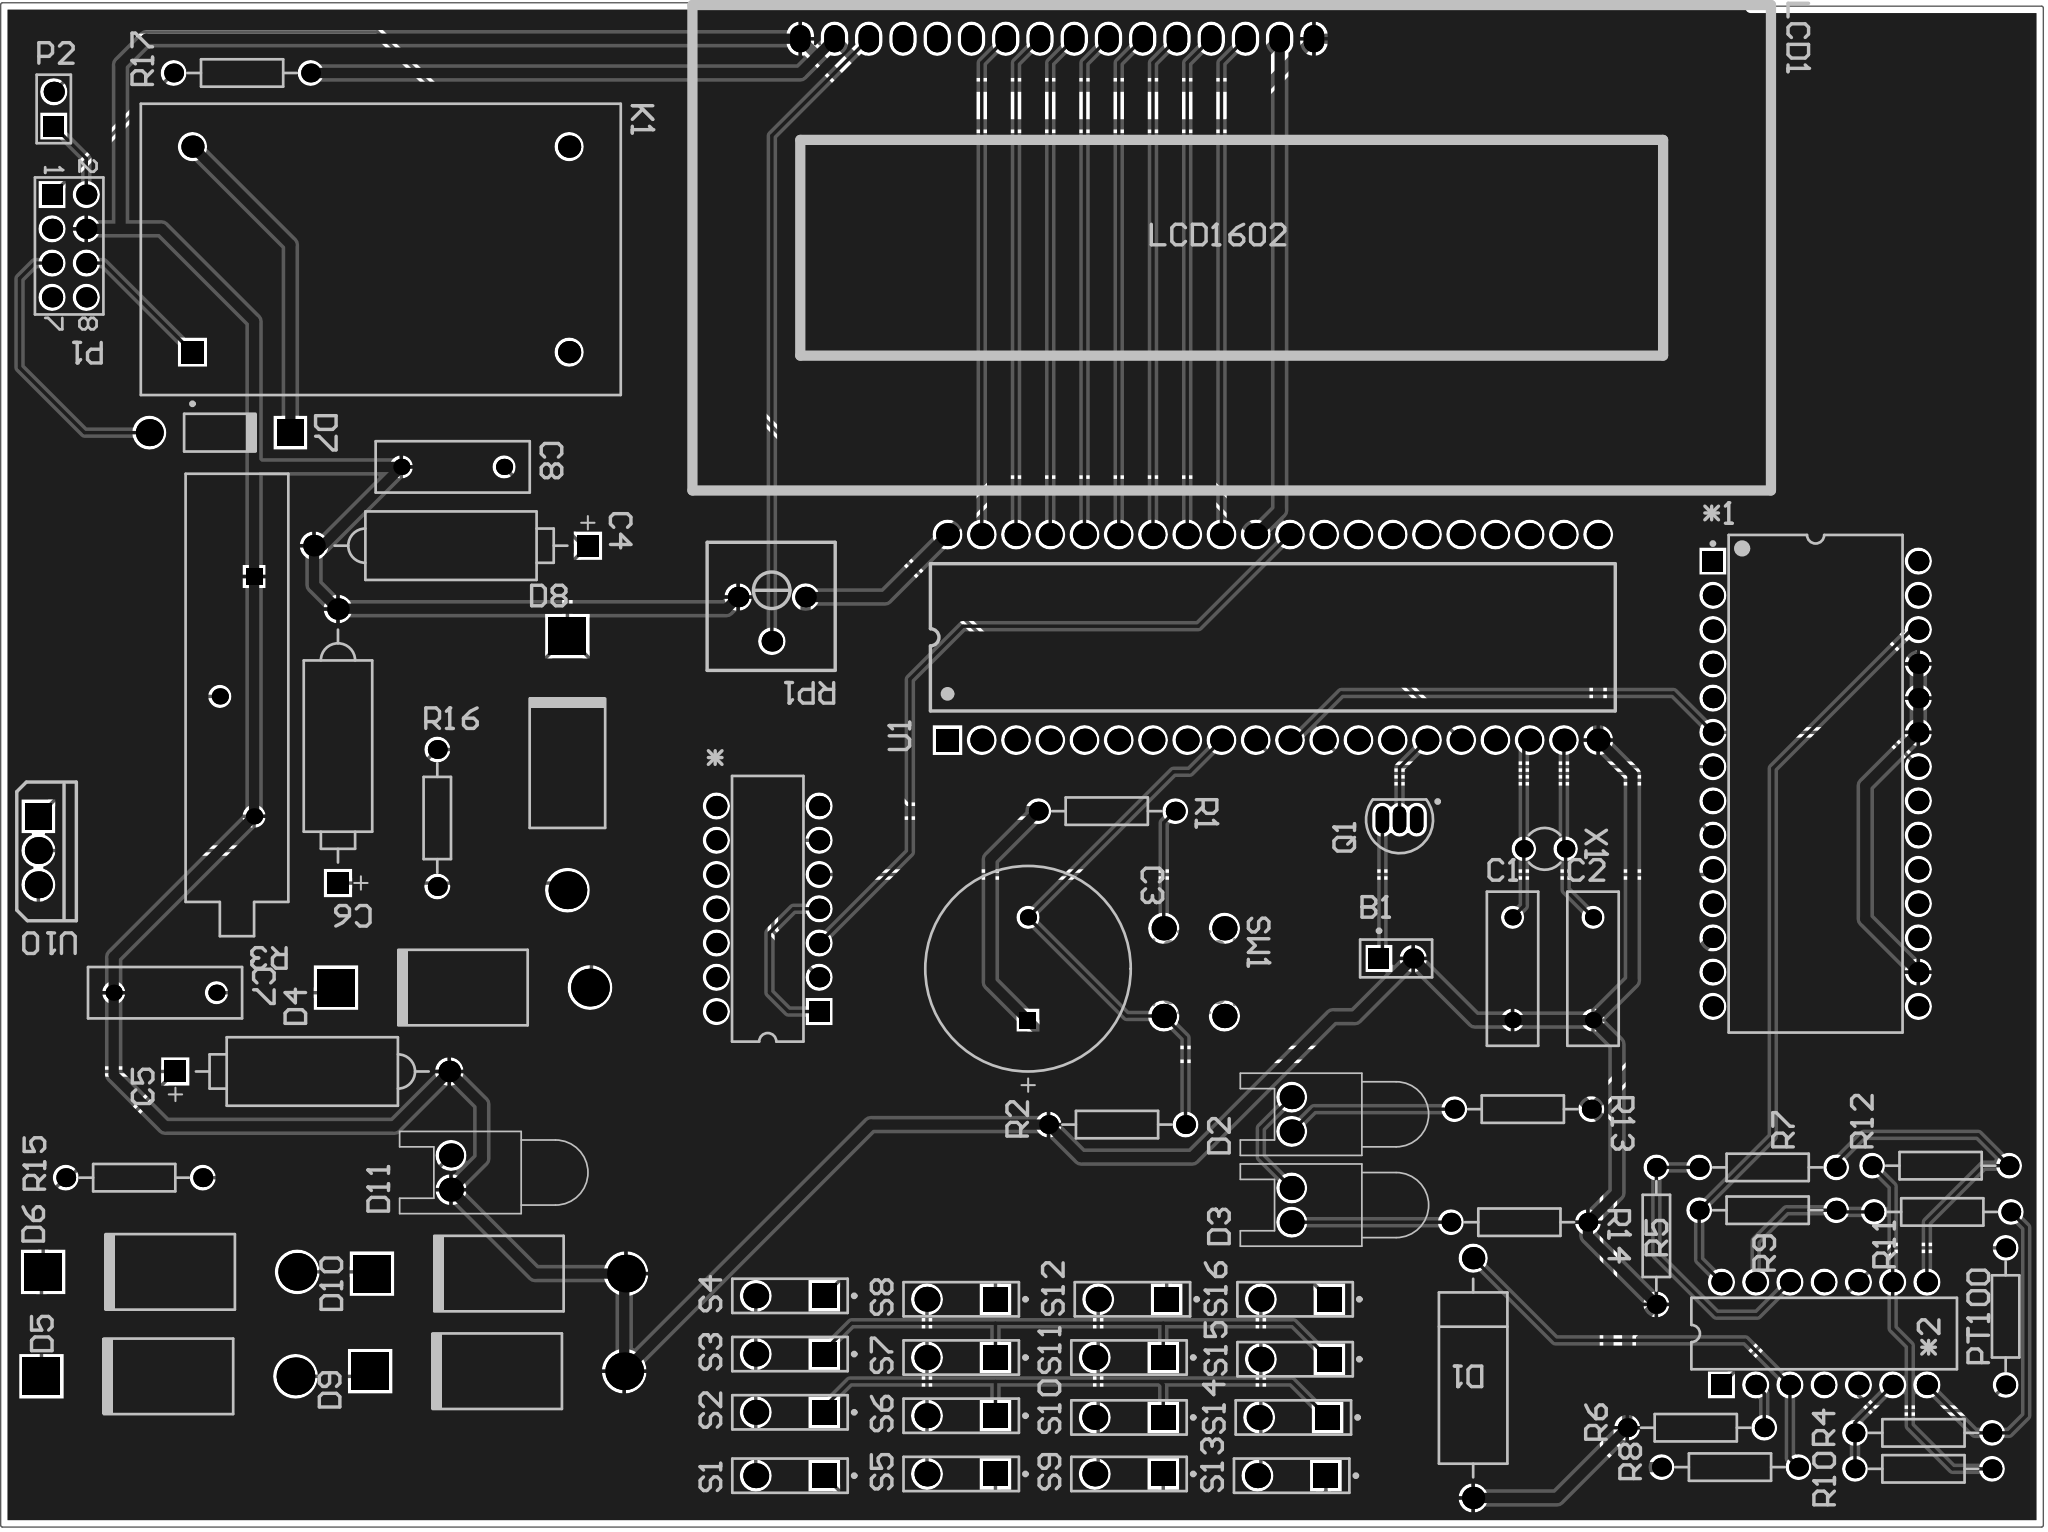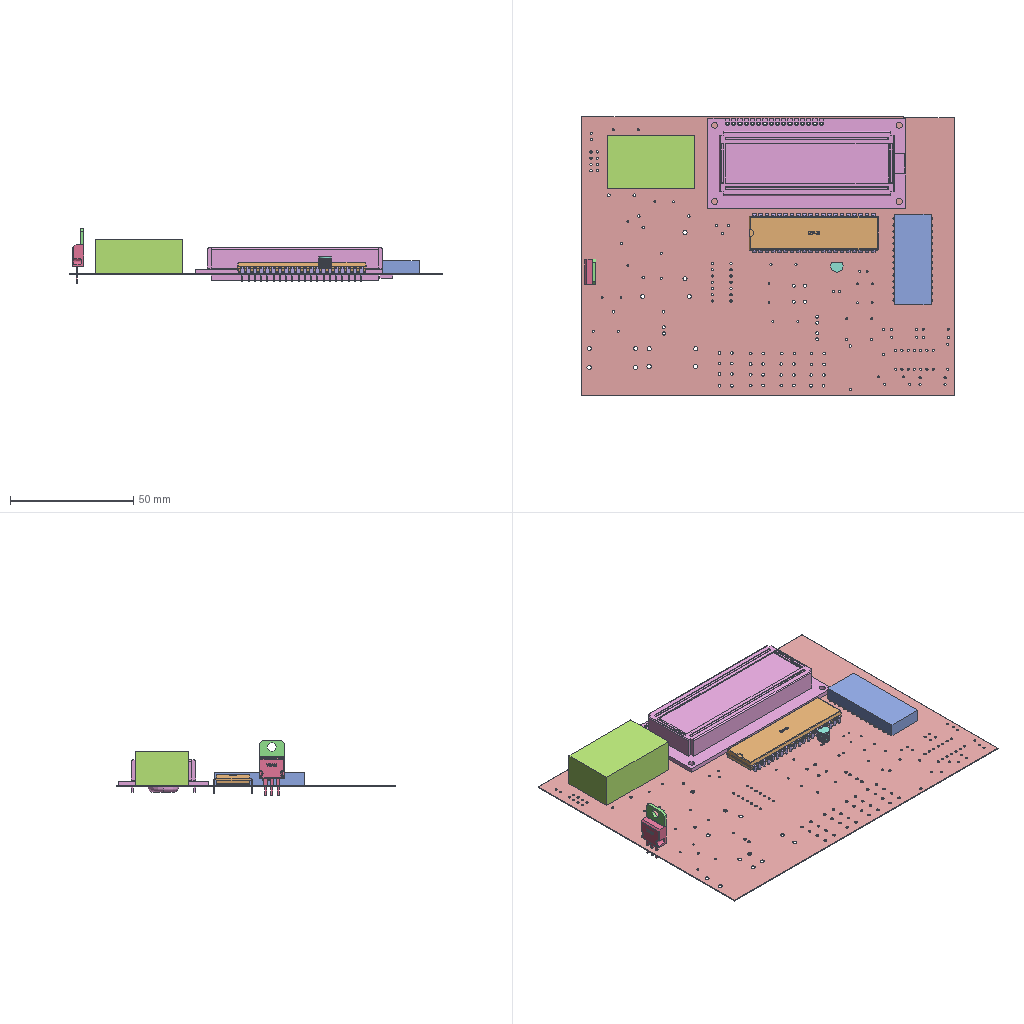Circuit board layout | Altium Designer | box 151.5 x 113 x 22.5 mm
Layer stack:
# Altium Designer layer stack of  (unit mm; dielectric type: 0 none, 1 core, 2 prepreg, 3 surface material)
index,name,kind,layer,copper_thickness_mm,dielectric_type,dielectric_thickness_mm,dielectric_material,dielectric_constant
0,Top Paste,other,,,,,,
1,Top Overlay,other,,,,,,
2,Top Solder,dielectric,,,3,0.0102,Solder Resist,3.5
3,Top Layer,copper,Top Layer,0.0356,,,,
4,Dielectric 1,dielectric,,,0,0.32,FR-4,4.8
5,Bottom Layer,copper,Bottom Layer,0.0356,,,,
6,Bottom Solder,dielectric,,,3,0.0102,Solder Resist,3.5
7,Bottom Overlay,other,,,,,,
8,Bottom Paste,other,,,,,,
# drill layer pairs: low layer,high layer
drill_pair,Top Layer,Bottom Layer
Part placement:
Designator,Comment,Layer,Footprint,Center-X(mm),Center-Y(mm),Rotation
*1,ADC0809,TopLayer,N28B,213.614,70.358,360
*2,LM324N,TopLayer,646-06,214.249,29.591,360
*,74LS74,TopLayer,646-06,135.89,61.087,90
B1,DC5V,TopLayer,PIN2,182.499,57.404,0
C1,104,TopLayer,RAD-0.3,191.135,56.642,90
C2,104,TopLayer,RAD-0.3,197.104,56.642,90
C3,10UF/16V,TopLayer,RB7.6-15,155.194,56.642,270
C4,Cap Pol2,TopLayer,POLAR0.8,112.395,88.011,360
C5,Cap Pol2,TopLayer,POLAR0.8,102.108,49.022,180
C6,Cap Pol2,TopLayer,POLAR0.8,104.013,73.152,270
C7,104,TopLayer,RAD-0.3,91.186,54.864,360
C8,104,TopLayer,RAD-0.3,112.522,93.853,360
D1,1N4733A,TopLayer,DIODE-0.7,188.214,26.289,90
D2,LED0,TopLayer,LED-0,174.752,45.847,90
D3,LED0,TopLayer,LED-0,174.752,39.116,90
D4,DIODE,TopLayer,DO-201AD,113.284,55.245,180
D5,DIODE,TopLayer,DO-201AD,91.44,26.416,180
D6,DIODE,TopLayer,DO-201AD,91.567,34.163,180
D7,Diode 1N4007,TopLayer,DO-41,95.25,96.393,360
D8,DIODE,TopLayer,DO-201AD,121.031,71.882,90
D9,DIODE,TopLayer,DO-201AD,115.824,26.797,180
D10,DIODE,TopLayer,DO-201AD,115.951,34.036,180
D11,LED0,TopLayer,LED-0,112.395,41.529,90
K1,Relay-SPST,TopLayer,MODULE4,107.188,109.982,360
LCD1,LCD 1602,TopLayer,LCD1602,157.353,125.603,360
P1,4N27,TopLayer,HDR2X4,84.074,110.236,270
P2,74F04,TopLayer,HDR1X2,82.931,120.396,90
PT100,30K,TopLayer,AXIAL-0.4,227.711,30.861,270
Q1,2N3906,TopLayer,TO-92A,182.753,67.691,90
R1,10K,TopLayer,AXIAL-0.4,161.036,68.326,360
R2,10K,TopLayer,AXIAL-0.4,161.798,45.085,180
R3,Res Tap,TopLayer,VR3,96.52,76.835,270
R4,450,TopLayer,AXIAL-0.4,221.615,22.225,180
R5,1K,TopLayer,AXIAL-0.4,201.803,36.83,90
R6,3.3K,TopLayer,AXIAL-0.4,204.724,22.606,180
R7,1K,TopLayer,AXIAL-0.4,210.058,41.91,360
R8,1K,TopLayer,AXIAL-0.4,207.264,19.685,180
R9,1K,TopLayer,AXIAL-0.4,210.058,38.735,360
R10,30K,TopLayer,AXIAL-0.4,221.615,19.558,360
R11,1K,TopLayer,AXIAL-0.4,223.012,38.608,180
R12,450,TopLayer,AXIAL-0.4,222.885,42.037,180
R13,250,TopLayer,AXIAL-0.4,191.897,46.228,360
R14,250,TopLayer,AXIAL-0.4,191.643,37.846,360
R15,30K,TopLayer,AXIAL-0.4,88.9,41.148,180
R16,200,TopLayer,AXIAL-0.4,111.379,67.818,90
R17,500,TopLayer,AXIAL-0.4,96.901,123.063,180
RP1,10K,TopLayer,电位器,136.195,82.563,180
S1,SW-PB,TopLayer,SPST-2,137.541,19.05,180
S2,SW-PB,TopLayer,SPST-2,137.541,23.749,180
S3,SW-PB,TopLayer,SPST-2,137.541,28.067,180
S4,SW-PB,TopLayer,SPST-2,137.541,32.385,180
S5,SW-PB,TopLayer,SPST-2,150.241,19.177,180
S6,SW-PB,TopLayer,SPST-2,150.241,23.495,180
S7,SW-PB,TopLayer,SPST-2,150.241,27.813,180
S8,SW-PB,TopLayer,SPST-2,150.241,32.131,180
S9,SW-PB,TopLayer,SPST-2,162.687,19.177,180
S10,SW-PB,TopLayer,SPST-2,162.687,23.368,180
S11,SW-PB,TopLayer,SPST-2,162.687,27.813,180
S12,SW-PB,TopLayer,SPST-2,162.941,32.131,180
S13,SW-PB,TopLayer,SPST-2,174.752,19.05,180
S14,SW-PB,TopLayer,SPST-2,174.879,23.368,180
S15,SW-PB,TopLayer,SPST-2,175.006,27.686,180
S16,SW-PB,TopLayer,SPST-2,175.006,32.131,180
SW1,6x6x5,TopLayer,四脚轻触开关,167.513,56.388,270
U1,STC89C5xx,TopLayer,DIP40,173.355,81.216,90
X1,12MHz,TopLayer,R38,193.522,65.532,270
U10,LM317,TopLayer,TO220A,81.788,65.405,270
Pad and via stacks:
# Altium Designer via and pad stacks of  (unit mm). Each distinct definition once, with the count of objects using it.
# via: kind,start_layer,end_layer,hole_mm,diameter_mm,mode(0 simple;1 top-mid-bottom;2 full stack),diameter_per_layer,count,example_net
# pad: kind,layer,hole_mm,hole_type(0 round;1 square;2 slot),plating,top_size,top_shape(1 round;2 rect;3 octagon;9 rounded rect),mid_size,bottom_size,mode,footprint,size_per_layer,count,example
pad,Multi-Layer,0.9,0,plated,1.5x1.5,1,1.5x1.5,1.5x1.5,0,HDR1X2,,1,P2.2
pad,Multi-Layer,0.9,0,plated,1.5x1.5,2,1.5x1.5,1.5x1.5,0,HDR1X2,,1,P2.1
pad,Multi-Layer,1.7,0,plated,2.8x2.8,1,2.8x2.8,2.8x2.8,0,DO-201AD,,6,D9.1
pad,Multi-Layer,1.7,0,plated,2.8x2.8,2,2.8x2.8,2.8x2.8,0,DO-201AD,,6,D9.2
pad,Multi-Layer,1.27,0,plated,1.778x1.778,1,1.778x1.778,1.778x1.778,0,LED-0,,6,D11.2
pad,Multi-Layer,1,0,plated,1.6x1.6,2,1.6x1.6,1.6x1.6,0,POLAR0.8,,3,C6.1
pad,Multi-Layer,1,0,plated,1.6x1.6,1,1.6x1.6,1.6x1.6,0,POLAR0.8,,3,C6.2
pad,Multi-Layer,0.7,0,plated,1.2x1.2,1,1.2x1.2,1.2x1.2,0,RAD-0.3,,8,C8.1
pad,Multi-Layer,0.7,0,plated,1.2x1.2,1,1.2x1.2,1.2x1.2,0,VR3,,2,R3.2
pad,Multi-Layer,0.7,0,plated,1.2x1.2,2,1.2x1.2,1.2x1.2,0,VR3,,1,R3.1
pad,Multi-Layer,1,0,plated,1.65x1.65,1,1.65x1.65,1.65x1.65,0,MODULE4,,3,K1.3
pad,Multi-Layer,1,0,plated,1.65x1.65,2,1.65x1.65,1.65x1.65,0,MODULE4,,1,K1.1
pad,Multi-Layer,0.85,0,plated,1.4x1.4,1,1.4x1.4,1.4x1.4,0,AXIAL-0.4,,34,R17.2
pad,Multi-Layer,0.9,0,plated,1.5x1.5,2,1.5x1.5,1.5x1.5,0,HDR2X4,,1,P1.1
pad,Multi-Layer,0.9,0,plated,1.5x1.5,1,1.5x1.5,1.5x1.5,0,HDR2X4,,7,P1.2
pad,Multi-Layer,1.2,0,plated,2x2,2,2x2,2x2,0,DO-41,,1,D7.2
pad,Multi-Layer,1.2,0,plated,2x2,1,2x2,2x2,0,DO-41,,1,D7.1
pad,Multi-Layer,0.9,0,plated,1.5x1.5,1,1.5x1.5,1.5x1.5,0,PIN2,,1,B1.2
pad,Multi-Layer,0.9,0,plated,1.5x1.5,2,1.5x1.5,1.5x1.5,0,PIN2,,1,B1.1
pad,Multi-Layer,0.9,0,plated,2x1,1,2x1,2x1,0,TO-92A,,3,Q1.1
pad,Multi-Layer,1,0,plated,1.65x1.65,1,1.65x1.65,1.65x1.65,0,DIODE-0.7,,2,D1.1
pad,Multi-Layer,1.1,0,plated,1.85x1.85,1,1.85x1.85,1.85x1.85,0,SPST-2,,16,S13.2
pad,Multi-Layer,1.1,0,plated,1.85x1.85,2,1.85x1.85,1.85x1.85,0,SPST-2,,16,S13.1
pad,Multi-Layer,0.9,0,plated,1.5x1.5,2,1.5x1.5,1.5x1.5,0,646-06,,2,*2.1
pad,Multi-Layer,0.9,0,plated,1.5x1.5,1,1.5x1.5,1.5x1.5,0,646-06,,26,*2.2
pad,Multi-Layer,0.7,0,plated,1.3x1.3,1,1.3x1.3,1.3x1.3,0,R38,,2,X1.2
pad,Multi-Layer,0.7,0,plated,1.2x1.2,1,1.2x1.2,1.2x1.2,0,RB7.6-15,,1,C3.2
pad,Multi-Layer,0.7,0,plated,1.2x1.2,2,1.2x1.2,1.2x1.2,0,RB7.6-15,,1,C3.1
pad,Multi-Layer,1.2,0,plated,1.8x1.8,1,1.8x1.8,1.8x1.8,0,\u00CB\u00C4\u00BD\u00C5\u00C7\u00E1\u00B4\u00A5\u00BF\u00AA\u00B9\u00D8,,4,SW1.1
pad,Multi-Layer,0.9,0,plated,1.5x1.5,2,1.5x1.5,1.5x1.5,0,N28B,,1,*1.1
pad,Multi-Layer,0.9,0,plated,1.5x1.5,1,1.5x1.5,1.5x1.5,0,N28B,,27,*1.2
pad,Multi-Layer,0.9,0,plated,1.524x1.524,1,1.524x1.524,1.524x1.524,0,\u00B5\u00E7\u00CE\u00BB\u00C6\u00F7,,3,RP1.3
pad,Multi-Layer,0.8,0,plated,1.7x1.7,2,1.7x1.7,1.7x1.7,0,DIP40,,1,U1.1
pad,Multi-Layer,0.8,0,plated,1.7x1.7,1,1.7x1.7,1.7x1.7,0,DIP40,,39,U1.2
pad,Multi-Layer,0.9,0,plated,1.524x2.032,1,1.524x2.032,1.524x2.032,0,LCD1602,,16,LCD1.6
pad,Multi-Layer,1.1,0,plated,2x2,2,2x2,2x2,0,TO220A,,1,U10.1
pad,Multi-Layer,1.1,0,plated,2x2,1,2x2,2x2,0,TO220A,,2,U10.3
Copper pours:
name,layer,net,type(0 solid;1 hatched;2 none)
Top Layer-No Net,Bottom Layer,GND,0
Top Layer-No Net,Top Layer,GND,0
Design rules, without the lines most boards share:
# Altium Designer design rules of  (exported by Altium Designer, unit mm)
# columns: name | kind | enabled | priority | scope1 | scope2 | descriptor | typed fields (field=value)
Clearance | 0 | enabled | 1 | All | All | Clearance Constraint (Gap=10mil) (All),(All) | gap=0.254
PlaneConnect | 6 | enabled | 1 | All | All | Power Plane Connect Rule(Relief Connect )(Expansion=20mil) (Conductor Width=10mil) (Air Gap=10mil) (Entries=4) (All) | relief_conductor_width=0.254 relief_entries=4 relief_expansion=0.508
PolygonConnect | 20 | enabled | 1 | All | All | Polygon Connect Rule(Relief Connect )(Conductor Width=10mil) (Relief Angle=90 Angle) (Entries=4) (Air Gap Width=10mil) (All),(All) | connect_style(0=relief,1=direct,2=none)=0 relief_conductor_width=0.254 relief_entries=4
Width | 2 | enabled | 1 | All | All | Width Constraint (Min=10mil) (Max=30mil) (Preferred=10mil) (All) |
RoutingVias | 11 | enabled | 1 | All | All | Routing Via (MinHoleWidth=28mil) (MaxHoleWidth=28mil) (PreferredHoleWidth=28mil) (MinWidth=50mil) (MaxWidth=50mil) (PreferedWidth=50mil) (All) | via_min_hole=0.7112 via_max_hole=0.7112 via_preferred_diameter=1.27 via_preferred_hole=0.7112
PasteMaskExpansion | 14 | enabled | 1 | All | All | Paste Mask Expansion (Expansion =0mil) (All) | expansion=0
SolderMaskExpansion | 13 | enabled | 1 | All | All | Solder Mask Expansion (Expansion =4mil) (All) | expansion=0.1016
DiffPairsRouting | 51 | enabled | 1 | All | All | Differential Pairs Uncoupled Length using the Gap Constraints (Min=10mil) (Max=10mil) (Prefered=10mil)  and Width Constraints (Min=15mil) (Max=15mil) (Prefered=15mil) (All) |
HoleToHoleClearance | 52 | enabled | 1 | All | All | Hole To Hole Clearance (Gap=10mil) (All),(All) | gap=0.254
MinimumSolderMaskSliver | 53 | enabled | 1 | All | All | Minimum Solder Mask Sliver (Gap=0mil) (All),(All) |
SilkToSolderMaskClearance | 54 | enabled | 1 | IsPad | All | Silk To Solder Mask (Clearance=0mil) (IsPad),(All) |
SilkToSilkClearance | 55 | enabled | 1 | All | All | Silk to Silk (Clearance=0mil) (All),(All) |